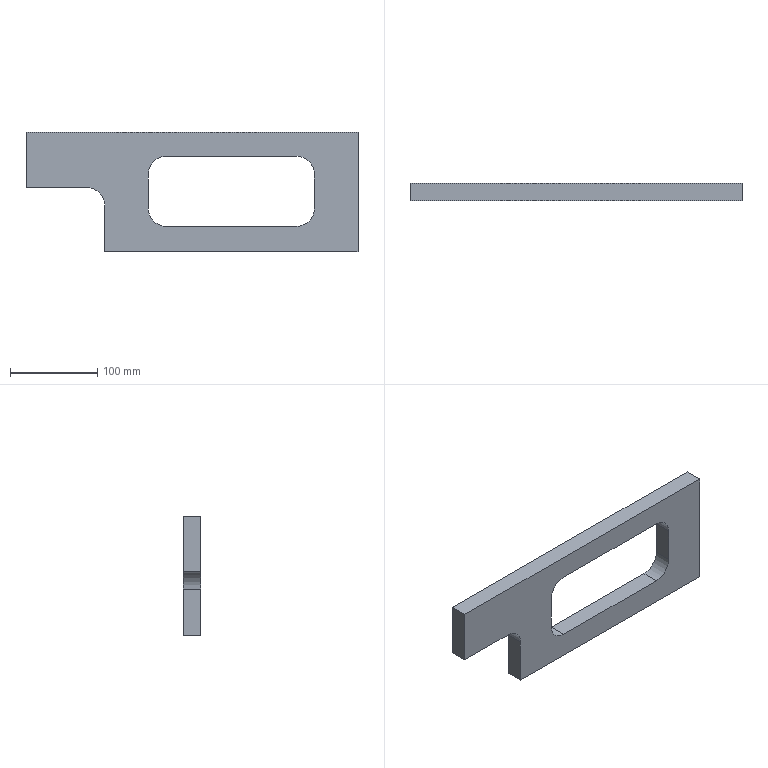Part | STEP file | Tube feed_id654_x_t | 1 solid | 17 faces | box 380 x 20 x 137 mm | volume 613484 mm3 | plane 12 | cylinder 5 | commonest cylinder face diameters 40 x5
STEP:
#1=CARTESIAN_POINT('',(0.,0.,0.));
#2=DIRECTION('',(0.,0.,1.));
#3=DIRECTION('',(1.,0.,0.));
#4=AXIS2_PLACEMENT_3D('',#1,#2,#3);
#5=CARTESIAN_POINT('',(206.,331.936,-108.75));
#6=VERTEX_POINT('',#5);
#7=CARTESIAN_POINT('',(206.,331.936,-68.75));
#8=VERTEX_POINT('',#7);
#9=CARTESIAN_POINT('',(206.,331.936,-48.75));
#10=DIRECTION('',(0.,0.,1.));
#11=VECTOR('',#10,1.);
#12=LINE('',#9,#11);
#13=CARTESIAN_POINT('',(206.,351.936,-48.75));
#14=DIRECTION('',(1.,0.,0.));
#15=DIRECTION('',(0.,0.,-1.));
#16=AXIS2_PLACEMENT_3D('',#13,#14,#15);
#17=PLANE('',#16);
#18=CARTESIAN_POINT('',(0.,-20.));
#19=DIRECTION('',(-1.,0.));
#20=VECTOR('',#19,1.);
#21=LINE('',#18,#20);
#22=(GEOMETRIC_REPRESENTATION_CONTEXT(2)PARAMETRIC_REPRESENTATION_CONTEXT()REPRESENTATION_CONTEXT('',''));
#23=DEFINITIONAL_REPRESENTATION('',(#21),#22);
#24=PCURVE('',#17,#23);
#25=CARTESIAN_POINT('',(0.,331.936,0.));
#26=DIRECTION('',(0.,-1.,0.));
#27=DIRECTION('',(0.,0.,1.));
#28=AXIS2_PLACEMENT_3D('',#25,#26,#27);
#29=PLANE('',#28);
#30=CARTESIAN_POINT('',(-48.75,-206.));
#31=DIRECTION('',(1.,0.));
#32=VECTOR('',#31,1.);
#33=LINE('',#30,#32);
#34=(GEOMETRIC_REPRESENTATION_CONTEXT(2)PARAMETRIC_REPRESENTATION_CONTEXT()REPRESENTATION_CONTEXT('',''));
#35=DEFINITIONAL_REPRESENTATION('',(#33),#34);
#36=PCURVE('',#29,#35);
#37=SURFACE_CURVE('',#12,(#24,#36),.PCURVE_S1.);
#38=EDGE_CURVE('',#6,#8,#37,.T.);
#39=ORIENTED_EDGE('',*,*,#38,.F.);
#40=CARTESIAN_POINT('',(206.,351.936,-108.75));
#41=VERTEX_POINT('',#40);
#42=CARTESIAN_POINT('',(206.,331.936,-108.75));
#43=DIRECTION('',(0.,1.,0.));
#44=VECTOR('',#43,1.);
#45=LINE('',#42,#44);
#46=CARTESIAN_POINT('',(60.,-20.));
#47=DIRECTION('',(0.,1.));
#48=VECTOR('',#47,1.);
#49=LINE('',#46,#48);
#50=(GEOMETRIC_REPRESENTATION_CONTEXT(2)PARAMETRIC_REPRESENTATION_CONTEXT()REPRESENTATION_CONTEXT('',''));
#51=DEFINITIONAL_REPRESENTATION('',(#49),#50);
#52=PCURVE('',#17,#51);
#53=CARTESIAN_POINT('',(226.,351.936,-108.75));
#54=DIRECTION('',(0.,1.,0.));
#55=DIRECTION('',(0.,0.,-1.));
#56=AXIS2_PLACEMENT_3D('',#53,#54,#55);
#57=CYLINDRICAL_SURFACE('',#56,20.);
#58=CARTESIAN_POINT('',(1.571,-20.));
#59=DIRECTION('',(0.,1.));
#60=VECTOR('',#59,1.);
#61=LINE('',#58,#60);
#62=(GEOMETRIC_REPRESENTATION_CONTEXT(2)PARAMETRIC_REPRESENTATION_CONTEXT()REPRESENTATION_CONTEXT('',''));
#63=DEFINITIONAL_REPRESENTATION('',(#61),#62);
#64=PCURVE('',#57,#63);
#65=SURFACE_CURVE('',#45,(#52,#64),.PCURVE_S1.);
#66=EDGE_CURVE('',#6,#41,#65,.T.);
#67=ORIENTED_EDGE('',*,*,#66,.T.);
#68=CARTESIAN_POINT('',(206.,351.936,-68.75));
#69=VERTEX_POINT('',#68);
#70=CARTESIAN_POINT('',(206.,351.936,-48.75));
#71=DIRECTION('',(0.,0.,1.));
#72=VECTOR('',#71,1.);
#73=LINE('',#70,#72);
#74=CARTESIAN_POINT('',(0.,0.));
#75=DIRECTION('',(-1.,0.));
#76=VECTOR('',#75,1.);
#77=LINE('',#74,#76);
#78=(GEOMETRIC_REPRESENTATION_CONTEXT(2)PARAMETRIC_REPRESENTATION_CONTEXT()REPRESENTATION_CONTEXT('',''));
#79=DEFINITIONAL_REPRESENTATION('',(#77),#78);
#80=PCURVE('',#17,#79);
#81=CARTESIAN_POINT('',(0.,351.936,0.));
#82=DIRECTION('',(0.,-1.,0.));
#83=DIRECTION('',(0.,0.,1.));
#84=AXIS2_PLACEMENT_3D('',#81,#82,#83);
#85=PLANE('',#84);
#86=CARTESIAN_POINT('',(-48.75,-206.));
#87=DIRECTION('',(1.,0.));
#88=VECTOR('',#87,1.);
#89=LINE('',#86,#88);
#90=(GEOMETRIC_REPRESENTATION_CONTEXT(2)PARAMETRIC_REPRESENTATION_CONTEXT()REPRESENTATION_CONTEXT('',''));
#91=DEFINITIONAL_REPRESENTATION('',(#89),#90);
#92=PCURVE('',#85,#91);
#93=SURFACE_CURVE('',#73,(#80,#92),.PCURVE_S1.);
#94=EDGE_CURVE('',#41,#69,#93,.T.);
#95=ORIENTED_EDGE('',*,*,#94,.T.);
#96=CARTESIAN_POINT('',(206.,351.936,-68.75));
#97=DIRECTION('',(0.,-1.,0.));
#98=VECTOR('',#97,1.);
#99=LINE('',#96,#98);
#100=CARTESIAN_POINT('',(20.,0.));
#101=DIRECTION('',(0.,-1.));
#102=VECTOR('',#101,1.);
#103=LINE('',#100,#102);
#104=(GEOMETRIC_REPRESENTATION_CONTEXT(2)PARAMETRIC_REPRESENTATION_CONTEXT()REPRESENTATION_CONTEXT('',''));
#105=DEFINITIONAL_REPRESENTATION('',(#103),#104);
#106=PCURVE('',#17,#105);
#107=CARTESIAN_POINT('',(226.,351.936,-68.75));
#108=DIRECTION('',(0.,1.,0.));
#109=DIRECTION('',(0.,0.,-1.));
#110=AXIS2_PLACEMENT_3D('',#107,#108,#109);
#111=CYLINDRICAL_SURFACE('',#110,20.);
#112=CARTESIAN_POINT('',(1.571,0.));
#113=DIRECTION('',(0.,-1.));
#114=VECTOR('',#113,1.);
#115=LINE('',#112,#114);
#116=(GEOMETRIC_REPRESENTATION_CONTEXT(2)PARAMETRIC_REPRESENTATION_CONTEXT()REPRESENTATION_CONTEXT('',''));
#117=DEFINITIONAL_REPRESENTATION('',(#115),#116);
#118=PCURVE('',#111,#117);
#119=SURFACE_CURVE('',#99,(#106,#118),.PCURVE_S1.);
#120=EDGE_CURVE('',#69,#8,#119,.T.);
#121=ORIENTED_EDGE('',*,*,#120,.T.);
#122=EDGE_LOOP('',(#39,#67,#95,#121));
#123=FACE_BOUND('',#122,.T.);
#124=ADVANCED_FACE('',(#123),#17,.T.);
#125=CARTESIAN_POINT('',(376.,351.936,-128.75));
#126=VERTEX_POINT('',#125);
#127=CARTESIAN_POINT('',(226.,351.936,-128.75));
#128=VERTEX_POINT('',#127);
#129=CARTESIAN_POINT('',(206.,351.936,-128.75));
#130=DIRECTION('',(-1.,0.,0.));
#131=VECTOR('',#130,1.);
#132=LINE('',#129,#131);
#133=CARTESIAN_POINT('',(206.,351.936,-128.75));
#134=DIRECTION('',(0.,0.,1.));
#135=DIRECTION('',(1.,0.,0.));
#136=AXIS2_PLACEMENT_3D('',#133,#134,#135);
#137=PLANE('',#136);
#138=CARTESIAN_POINT('',(0.,0.));
#139=DIRECTION('',(-1.,0.));
#140=VECTOR('',#139,1.);
#141=LINE('',#138,#140);
#142=(GEOMETRIC_REPRESENTATION_CONTEXT(2)PARAMETRIC_REPRESENTATION_CONTEXT()REPRESENTATION_CONTEXT('',''));
#143=DEFINITIONAL_REPRESENTATION('',(#141),#142);
#144=PCURVE('',#137,#143);
#145=CARTESIAN_POINT('',(-128.75,-206.));
#146=DIRECTION('',(0.,1.));
#147=VECTOR('',#146,1.);
#148=LINE('',#145,#147);
#149=(GEOMETRIC_REPRESENTATION_CONTEXT(2)PARAMETRIC_REPRESENTATION_CONTEXT()REPRESENTATION_CONTEXT('',''));
#150=DEFINITIONAL_REPRESENTATION('',(#148),#149);
#151=PCURVE('',#85,#150);
#152=SURFACE_CURVE('',#132,(#144,#151),.PCURVE_S1.);
#153=EDGE_CURVE('',#126,#128,#152,.T.);
#154=ORIENTED_EDGE('',*,*,#153,.T.);
#155=CARTESIAN_POINT('',(226.,331.936,-128.75));
#156=VERTEX_POINT('',#155);
#157=CARTESIAN_POINT('',(226.,351.936,-128.75));
#158=DIRECTION('',(0.,-1.,0.));
#159=VECTOR('',#158,1.);
#160=LINE('',#157,#159);
#161=CARTESIAN_POINT('',(20.,0.));
#162=DIRECTION('',(0.,-1.));
#163=VECTOR('',#162,1.);
#164=LINE('',#161,#163);
#165=(GEOMETRIC_REPRESENTATION_CONTEXT(2)PARAMETRIC_REPRESENTATION_CONTEXT()REPRESENTATION_CONTEXT('',''));
#166=DEFINITIONAL_REPRESENTATION('',(#164),#165);
#167=PCURVE('',#137,#166);
#168=CARTESIAN_POINT('',(0.,0.));
#169=DIRECTION('',(0.,-1.));
#170=VECTOR('',#169,1.);
#171=LINE('',#168,#170);
#172=(GEOMETRIC_REPRESENTATION_CONTEXT(2)PARAMETRIC_REPRESENTATION_CONTEXT()REPRESENTATION_CONTEXT('',''));
#173=DEFINITIONAL_REPRESENTATION('',(#171),#172);
#174=PCURVE('',#57,#173);
#175=SURFACE_CURVE('',#160,(#167,#174),.PCURVE_S1.);
#176=EDGE_CURVE('',#128,#156,#175,.T.);
#177=ORIENTED_EDGE('',*,*,#176,.T.);
#178=CARTESIAN_POINT('',(376.,331.936,-128.75));
#179=VERTEX_POINT('',#178);
#180=CARTESIAN_POINT('',(206.,331.936,-128.75));
#181=DIRECTION('',(-1.,0.,0.));
#182=VECTOR('',#181,1.);
#183=LINE('',#180,#182);
#184=CARTESIAN_POINT('',(0.,-20.));
#185=DIRECTION('',(-1.,0.));
#186=VECTOR('',#185,1.);
#187=LINE('',#184,#186);
#188=(GEOMETRIC_REPRESENTATION_CONTEXT(2)PARAMETRIC_REPRESENTATION_CONTEXT()REPRESENTATION_CONTEXT('',''));
#189=DEFINITIONAL_REPRESENTATION('',(#187),#188);
#190=PCURVE('',#137,#189);
#191=CARTESIAN_POINT('',(-128.75,-206.));
#192=DIRECTION('',(0.,1.));
#193=VECTOR('',#192,1.);
#194=LINE('',#191,#193);
#195=(GEOMETRIC_REPRESENTATION_CONTEXT(2)PARAMETRIC_REPRESENTATION_CONTEXT()REPRESENTATION_CONTEXT('',''));
#196=DEFINITIONAL_REPRESENTATION('',(#194),#195);
#197=PCURVE('',#29,#196);
#198=SURFACE_CURVE('',#183,(#190,#197),.PCURVE_S1.);
#199=EDGE_CURVE('',#179,#156,#198,.T.);
#200=ORIENTED_EDGE('',*,*,#199,.F.);
#201=CARTESIAN_POINT('',(376.,331.936,-128.75));
#202=DIRECTION('',(0.,1.,0.));
#203=VECTOR('',#202,1.);
#204=LINE('',#201,#203);
#205=CARTESIAN_POINT('',(170.,-20.));
#206=DIRECTION('',(0.,1.));
#207=VECTOR('',#206,1.);
#208=LINE('',#205,#207);
#209=(GEOMETRIC_REPRESENTATION_CONTEXT(2)PARAMETRIC_REPRESENTATION_CONTEXT()REPRESENTATION_CONTEXT('',''));
#210=DEFINITIONAL_REPRESENTATION('',(#208),#209);
#211=PCURVE('',#137,#210);
#212=CARTESIAN_POINT('',(376.,351.936,-108.75));
#213=DIRECTION('',(0.,1.,0.));
#214=DIRECTION('',(0.,0.,-1.));
#215=AXIS2_PLACEMENT_3D('',#212,#213,#214);
#216=CYLINDRICAL_SURFACE('',#215,20.);
#217=CARTESIAN_POINT('',(6.283,-20.));
#218=DIRECTION('',(0.,1.));
#219=VECTOR('',#218,1.);
#220=LINE('',#217,#219);
#221=(GEOMETRIC_REPRESENTATION_CONTEXT(2)PARAMETRIC_REPRESENTATION_CONTEXT()REPRESENTATION_CONTEXT('',''));
#222=DEFINITIONAL_REPRESENTATION('',(#220),#221);
#223=PCURVE('',#216,#222);
#224=SURFACE_CURVE('',#204,(#211,#223),.PCURVE_S1.);
#225=EDGE_CURVE('',#179,#126,#224,.T.);
#226=ORIENTED_EDGE('',*,*,#225,.T.);
#227=EDGE_LOOP('',(#154,#177,#200,#226));
#228=FACE_BOUND('',#227,.T.);
#229=ADVANCED_FACE('',(#228),#137,.T.);
#230=CARTESIAN_POINT('',(396.,331.936,-68.75));
#231=VERTEX_POINT('',#230);
#232=CARTESIAN_POINT('',(396.,331.936,-108.75));
#233=VERTEX_POINT('',#232);
#234=CARTESIAN_POINT('',(396.,331.936,-128.75));
#235=DIRECTION('',(0.,0.,-1.));
#236=VECTOR('',#235,1.);
#237=LINE('',#234,#236);
#238=CARTESIAN_POINT('',(396.,351.936,-128.75));
#239=DIRECTION('',(-1.,0.,0.));
#240=DIRECTION('',(0.,0.,1.));
#241=AXIS2_PLACEMENT_3D('',#238,#239,#240);
#242=PLANE('',#241);
#243=CARTESIAN_POINT('',(0.,-20.));
#244=DIRECTION('',(-1.,0.));
#245=VECTOR('',#244,1.);
#246=LINE('',#243,#245);
#247=(GEOMETRIC_REPRESENTATION_CONTEXT(2)PARAMETRIC_REPRESENTATION_CONTEXT()REPRESENTATION_CONTEXT('',''));
#248=DEFINITIONAL_REPRESENTATION('',(#246),#247);
#249=PCURVE('',#242,#248);
#250=CARTESIAN_POINT('',(-128.75,-396.));
#251=DIRECTION('',(-1.,0.));
#252=VECTOR('',#251,1.);
#253=LINE('',#250,#252);
#254=(GEOMETRIC_REPRESENTATION_CONTEXT(2)PARAMETRIC_REPRESENTATION_CONTEXT()REPRESENTATION_CONTEXT('',''));
#255=DEFINITIONAL_REPRESENTATION('',(#253),#254);
#256=PCURVE('',#29,#255);
#257=SURFACE_CURVE('',#237,(#249,#256),.PCURVE_S1.);
#258=EDGE_CURVE('',#231,#233,#257,.T.);
#259=ORIENTED_EDGE('',*,*,#258,.F.);
#260=CARTESIAN_POINT('',(396.,351.936,-68.75));
#261=VERTEX_POINT('',#260);
#262=CARTESIAN_POINT('',(396.,331.936,-68.75));
#263=DIRECTION('',(0.,1.,0.));
#264=VECTOR('',#263,1.);
#265=LINE('',#262,#264);
#266=CARTESIAN_POINT('',(60.,-20.));
#267=DIRECTION('',(0.,1.));
#268=VECTOR('',#267,1.);
#269=LINE('',#266,#268);
#270=(GEOMETRIC_REPRESENTATION_CONTEXT(2)PARAMETRIC_REPRESENTATION_CONTEXT()REPRESENTATION_CONTEXT('',''));
#271=DEFINITIONAL_REPRESENTATION('',(#269),#270);
#272=PCURVE('',#242,#271);
#273=CARTESIAN_POINT('',(376.,351.936,-68.75));
#274=DIRECTION('',(0.,1.,0.));
#275=DIRECTION('',(0.,0.,-1.));
#276=AXIS2_PLACEMENT_3D('',#273,#274,#275);
#277=CYLINDRICAL_SURFACE('',#276,20.);
#278=CARTESIAN_POINT('',(4.712,-20.));
#279=DIRECTION('',(0.,1.));
#280=VECTOR('',#279,1.);
#281=LINE('',#278,#280);
#282=(GEOMETRIC_REPRESENTATION_CONTEXT(2)PARAMETRIC_REPRESENTATION_CONTEXT()REPRESENTATION_CONTEXT('',''));
#283=DEFINITIONAL_REPRESENTATION('',(#281),#282);
#284=PCURVE('',#277,#283);
#285=SURFACE_CURVE('',#265,(#272,#284),.PCURVE_S1.);
#286=EDGE_CURVE('',#231,#261,#285,.T.);
#287=ORIENTED_EDGE('',*,*,#286,.T.);
#288=CARTESIAN_POINT('',(396.,351.936,-108.75));
#289=VERTEX_POINT('',#288);
#290=CARTESIAN_POINT('',(396.,351.936,-128.75));
#291=DIRECTION('',(0.,0.,-1.));
#292=VECTOR('',#291,1.);
#293=LINE('',#290,#292);
#294=CARTESIAN_POINT('',(0.,0.));
#295=DIRECTION('',(-1.,0.));
#296=VECTOR('',#295,1.);
#297=LINE('',#294,#296);
#298=(GEOMETRIC_REPRESENTATION_CONTEXT(2)PARAMETRIC_REPRESENTATION_CONTEXT()REPRESENTATION_CONTEXT('',''));
#299=DEFINITIONAL_REPRESENTATION('',(#297),#298);
#300=PCURVE('',#242,#299);
#301=CARTESIAN_POINT('',(-128.75,-396.));
#302=DIRECTION('',(-1.,0.));
#303=VECTOR('',#302,1.);
#304=LINE('',#301,#303);
#305=(GEOMETRIC_REPRESENTATION_CONTEXT(2)PARAMETRIC_REPRESENTATION_CONTEXT()REPRESENTATION_CONTEXT('',''));
#306=DEFINITIONAL_REPRESENTATION('',(#304),#305);
#307=PCURVE('',#85,#306);
#308=SURFACE_CURVE('',#293,(#300,#307),.PCURVE_S1.);
#309=EDGE_CURVE('',#261,#289,#308,.T.);
#310=ORIENTED_EDGE('',*,*,#309,.T.);
#311=CARTESIAN_POINT('',(396.,351.936,-108.75));
#312=DIRECTION('',(0.,-1.,0.));
#313=VECTOR('',#312,1.);
#314=LINE('',#311,#313);
#315=CARTESIAN_POINT('',(20.,0.));
#316=DIRECTION('',(0.,-1.));
#317=VECTOR('',#316,1.);
#318=LINE('',#315,#317);
#319=(GEOMETRIC_REPRESENTATION_CONTEXT(2)PARAMETRIC_REPRESENTATION_CONTEXT()REPRESENTATION_CONTEXT('',''));
#320=DEFINITIONAL_REPRESENTATION('',(#318),#319);
#321=PCURVE('',#242,#320);
#322=CARTESIAN_POINT('',(4.712,0.));
#323=DIRECTION('',(0.,-1.));
#324=VECTOR('',#323,1.);
#325=LINE('',#322,#324);
#326=(GEOMETRIC_REPRESENTATION_CONTEXT(2)PARAMETRIC_REPRESENTATION_CONTEXT()REPRESENTATION_CONTEXT('',''));
#327=DEFINITIONAL_REPRESENTATION('',(#325),#326);
#328=PCURVE('',#216,#327);
#329=SURFACE_CURVE('',#314,(#321,#328),.PCURVE_S1.);
#330=EDGE_CURVE('',#289,#233,#329,.T.);
#331=ORIENTED_EDGE('',*,*,#330,.T.);
#332=EDGE_LOOP('',(#259,#287,#310,#331));
#333=FACE_BOUND('',#332,.T.);
#334=ADVANCED_FACE('',(#333),#242,.T.);
#335=CARTESIAN_POINT('',(66.,331.936,-21.));
#336=VERTEX_POINT('',#335);
#337=CARTESIAN_POINT('',(66.,331.936,-84.5));
#338=VERTEX_POINT('',#337);
#339=CARTESIAN_POINT('',(66.,331.936,-84.5));
#340=DIRECTION('',(0.,0.,-1.));
#341=VECTOR('',#340,1.);
#342=LINE('',#339,#341);
#343=CARTESIAN_POINT('',(66.,351.936,-84.5));
#344=DIRECTION('',(-1.,0.,0.));
#345=DIRECTION('',(0.,0.,1.));
#346=AXIS2_PLACEMENT_3D('',#343,#344,#345);
#347=PLANE('',#346);
#348=CARTESIAN_POINT('',(0.,-20.));
#349=DIRECTION('',(-1.,0.));
#350=VECTOR('',#349,1.);
#351=LINE('',#348,#350);
#352=(GEOMETRIC_REPRESENTATION_CONTEXT(2)PARAMETRIC_REPRESENTATION_CONTEXT()REPRESENTATION_CONTEXT('',''));
#353=DEFINITIONAL_REPRESENTATION('',(#351),#352);
#354=PCURVE('',#347,#353);
#355=CARTESIAN_POINT('',(-84.5,-66.));
#356=DIRECTION('',(-1.,0.));
#357=VECTOR('',#356,1.);
#358=LINE('',#355,#357);
#359=(GEOMETRIC_REPRESENTATION_CONTEXT(2)PARAMETRIC_REPRESENTATION_CONTEXT()REPRESENTATION_CONTEXT('',''));
#360=DEFINITIONAL_REPRESENTATION('',(#358),#359);
#361=PCURVE('',#29,#360);
#362=SURFACE_CURVE('',#342,(#354,#361),.PCURVE_S1.);
#363=EDGE_CURVE('',#336,#338,#362,.T.);
#364=ORIENTED_EDGE('',*,*,#363,.F.);
#365=CARTESIAN_POINT('',(66.,351.936,-21.));
#366=VERTEX_POINT('',#365);
#367=CARTESIAN_POINT('',(66.,351.936,-21.));
#368=DIRECTION('',(0.,1.,0.));
#369=VECTOR('',#368,1.);
#370=LINE('',#367,#369);
#371=CARTESIAN_POINT('',(63.5,0.));
#372=DIRECTION('',(0.,1.));
#373=VECTOR('',#372,1.);
#374=LINE('',#371,#373);
#375=(GEOMETRIC_REPRESENTATION_CONTEXT(2)PARAMETRIC_REPRESENTATION_CONTEXT()REPRESENTATION_CONTEXT('',''));
#376=DEFINITIONAL_REPRESENTATION('',(#374),#375);
#377=PCURVE('',#347,#376);
#378=CARTESIAN_POINT('',(66.,351.936,-21.));
#379=DIRECTION('',(0.,0.,1.));
#380=DIRECTION('',(1.,0.,0.));
#381=AXIS2_PLACEMENT_3D('',#378,#379,#380);
#382=PLANE('',#381);
#383=CARTESIAN_POINT('',(0.,0.));
#384=DIRECTION('',(0.,1.));
#385=VECTOR('',#384,1.);
#386=LINE('',#383,#385);
#387=(GEOMETRIC_REPRESENTATION_CONTEXT(2)PARAMETRIC_REPRESENTATION_CONTEXT()REPRESENTATION_CONTEXT('',''));
#388=DEFINITIONAL_REPRESENTATION('',(#386),#387);
#389=PCURVE('',#382,#388);
#390=SURFACE_CURVE('',#370,(#377,#389),.PCURVE_S1.);
#391=EDGE_CURVE('',#336,#366,#390,.T.);
#392=ORIENTED_EDGE('',*,*,#391,.T.);
#393=CARTESIAN_POINT('',(66.,351.936,-84.5));
#394=VERTEX_POINT('',#393);
#395=CARTESIAN_POINT('',(66.,351.936,-84.5));
#396=DIRECTION('',(0.,0.,-1.));
#397=VECTOR('',#396,1.);
#398=LINE('',#395,#397);
#399=CARTESIAN_POINT('',(0.,0.));
#400=DIRECTION('',(-1.,0.));
#401=VECTOR('',#400,1.);
#402=LINE('',#399,#401);
#403=(GEOMETRIC_REPRESENTATION_CONTEXT(2)PARAMETRIC_REPRESENTATION_CONTEXT()REPRESENTATION_CONTEXT('',''));
#404=DEFINITIONAL_REPRESENTATION('',(#402),#403);
#405=PCURVE('',#347,#404);
#406=CARTESIAN_POINT('',(-84.5,-66.));
#407=DIRECTION('',(-1.,0.));
#408=VECTOR('',#407,1.);
#409=LINE('',#406,#408);
#410=(GEOMETRIC_REPRESENTATION_CONTEXT(2)PARAMETRIC_REPRESENTATION_CONTEXT()REPRESENTATION_CONTEXT('',''));
#411=DEFINITIONAL_REPRESENTATION('',(#409),#410);
#412=PCURVE('',#85,#411);
#413=SURFACE_CURVE('',#398,(#405,#412),.PCURVE_S1.);
#414=EDGE_CURVE('',#366,#394,#413,.T.);
#415=ORIENTED_EDGE('',*,*,#414,.T.);
#416=CARTESIAN_POINT('',(66.,351.936,-84.5));
#417=DIRECTION('',(0.,1.,0.));
#418=VECTOR('',#417,1.);
#419=LINE('',#416,#418);
#420=CARTESIAN_POINT('',(0.,0.));
#421=DIRECTION('',(0.,1.));
#422=VECTOR('',#421,1.);
#423=LINE('',#420,#422);
#424=(GEOMETRIC_REPRESENTATION_CONTEXT(2)PARAMETRIC_REPRESENTATION_CONTEXT()REPRESENTATION_CONTEXT('',''));
#425=DEFINITIONAL_REPRESENTATION('',(#423),#424);
#426=PCURVE('',#347,#425);
#427=CARTESIAN_POINT('',(156.,351.936,-84.5));
#428=DIRECTION('',(0.,0.,-1.));
#429=DIRECTION('',(-1.,0.,0.));
#430=AXIS2_PLACEMENT_3D('',#427,#428,#429);
#431=PLANE('',#430);
#432=CARTESIAN_POINT('',(90.,0.));
#433=DIRECTION('',(0.,1.));
#434=VECTOR('',#433,1.);
#435=LINE('',#432,#434);
#436=(GEOMETRIC_REPRESENTATION_CONTEXT(2)PARAMETRIC_REPRESENTATION_CONTEXT()REPRESENTATION_CONTEXT('',''));
#437=DEFINITIONAL_REPRESENTATION('',(#435),#436);
#438=PCURVE('',#431,#437);
#439=SURFACE_CURVE('',#419,(#426,#438),.PCURVE_S1.);
#440=EDGE_CURVE('',#338,#394,#439,.T.);
#441=ORIENTED_EDGE('',*,*,#440,.F.);
#442=EDGE_LOOP('',(#364,#392,#415,#441));
#443=FACE_BOUND('',#442,.T.);
#444=ADVANCED_FACE('',(#443),#347,.T.);
#445=CARTESIAN_POINT('',(446.,331.936,-21.));
#446=VERTEX_POINT('',#445);
#447=CARTESIAN_POINT('',(0.,331.936,-21.));
#448=DIRECTION('',(-1.,0.,0.));
#449=VECTOR('',#448,1.);
#450=LINE('',#447,#449);
#451=CARTESIAN_POINT('',(-66.,-20.));
#452=DIRECTION('',(-1.,0.));
#453=VECTOR('',#452,1.);
#454=LINE('',#451,#453);
#455=(GEOMETRIC_REPRESENTATION_CONTEXT(2)PARAMETRIC_REPRESENTATION_CONTEXT()REPRESENTATION_CONTEXT('',''));
#456=DEFINITIONAL_REPRESENTATION('',(#454),#455);
#457=PCURVE('',#382,#456);
#458=CARTESIAN_POINT('',(-21.,0.));
#459=DIRECTION('',(0.,1.));
#460=VECTOR('',#459,1.);
#461=LINE('',#458,#460);
#462=(GEOMETRIC_REPRESENTATION_CONTEXT(2)PARAMETRIC_REPRESENTATION_CONTEXT()REPRESENTATION_CONTEXT('',''));
#463=DEFINITIONAL_REPRESENTATION('',(#461),#462);
#464=PCURVE('',#29,#463);
#465=SURFACE_CURVE('',#450,(#457,#464),.PCURVE_S1.);
#466=EDGE_CURVE('',#446,#336,#465,.T.);
#467=ORIENTED_EDGE('',*,*,#466,.F.);
#468=CARTESIAN_POINT('',(446.,351.936,-21.));
#469=VERTEX_POINT('',#468);
#470=CARTESIAN_POINT('',(446.,351.936,-21.));
#471=DIRECTION('',(0.,1.,0.));
#472=VECTOR('',#471,1.);
#473=LINE('',#470,#472);
#474=CARTESIAN_POINT('',(380.,0.));
#475=DIRECTION('',(0.,1.));
#476=VECTOR('',#475,1.);
#477=LINE('',#474,#476);
#478=(GEOMETRIC_REPRESENTATION_CONTEXT(2)PARAMETRIC_REPRESENTATION_CONTEXT()REPRESENTATION_CONTEXT('',''));
#479=DEFINITIONAL_REPRESENTATION('',(#477),#478);
#480=PCURVE('',#382,#479);
#481=CARTESIAN_POINT('',(446.,351.936,-19.5));
#482=DIRECTION('',(1.,0.,0.));
#483=DIRECTION('',(0.,0.,-1.));
#484=AXIS2_PLACEMENT_3D('',#481,#482,#483);
#485=PLANE('',#484);
#486=CARTESIAN_POINT('',(1.5,0.));
#487=DIRECTION('',(0.,1.));
#488=VECTOR('',#487,1.);
#489=LINE('',#486,#488);
#490=(GEOMETRIC_REPRESENTATION_CONTEXT(2)PARAMETRIC_REPRESENTATION_CONTEXT()REPRESENTATION_CONTEXT('',''));
#491=DEFINITIONAL_REPRESENTATION('',(#489),#490);
#492=PCURVE('',#485,#491);
#493=SURFACE_CURVE('',#473,(#480,#492),.PCURVE_S1.);
#494=EDGE_CURVE('',#446,#469,#493,.T.);
#495=ORIENTED_EDGE('',*,*,#494,.T.);
#496=CARTESIAN_POINT('',(0.,351.936,-21.));
#497=DIRECTION('',(-1.,0.,0.));
#498=VECTOR('',#497,1.);
#499=LINE('',#496,#498);
#500=CARTESIAN_POINT('',(-66.,0.));
#501=DIRECTION('',(-1.,0.));
#502=VECTOR('',#501,1.);
#503=LINE('',#500,#502);
#504=(GEOMETRIC_REPRESENTATION_CONTEXT(2)PARAMETRIC_REPRESENTATION_CONTEXT()REPRESENTATION_CONTEXT('',''));
#505=DEFINITIONAL_REPRESENTATION('',(#503),#504);
#506=PCURVE('',#382,#505);
#507=CARTESIAN_POINT('',(-21.,0.));
#508=DIRECTION('',(0.,1.));
#509=VECTOR('',#508,1.);
#510=LINE('',#507,#509);
#511=(GEOMETRIC_REPRESENTATION_CONTEXT(2)PARAMETRIC_REPRESENTATION_CONTEXT()REPRESENTATION_CONTEXT('',''));
#512=DEFINITIONAL_REPRESENTATION('',(#510),#511);
#513=PCURVE('',#85,#512);
#514=SURFACE_CURVE('',#499,(#506,#513),.PCURVE_S1.);
#515=EDGE_CURVE('',#469,#366,#514,.T.);
#516=ORIENTED_EDGE('',*,*,#515,.T.);
#517=ORIENTED_EDGE('',*,*,#391,.F.);
#518=EDGE_LOOP('',(#467,#495,#516,#517));
#519=FACE_BOUND('',#518,.T.);
#520=ADVANCED_FACE('',(#519),#382,.T.);
#521=CARTESIAN_POINT('',(446.,331.936,-158.));
#522=VERTEX_POINT('',#521);
#523=CARTESIAN_POINT('',(446.,331.936,-19.5));
#524=DIRECTION('',(0.,0.,1.));
#525=VECTOR('',#524,1.);
#526=LINE('',#523,#525);
#527=CARTESIAN_POINT('',(0.,-20.));
#528=DIRECTION('',(-1.,0.));
#529=VECTOR('',#528,1.);
#530=LINE('',#527,#529);
#531=(GEOMETRIC_REPRESENTATION_CONTEXT(2)PARAMETRIC_REPRESENTATION_CONTEXT()REPRESENTATION_CONTEXT('',''));
#532=DEFINITIONAL_REPRESENTATION('',(#530),#531);
#533=PCURVE('',#485,#532);
#534=CARTESIAN_POINT('',(-19.5,-446.));
#535=DIRECTION('',(1.,0.));
#536=VECTOR('',#535,1.);
#537=LINE('',#534,#536);
#538=(GEOMETRIC_REPRESENTATION_CONTEXT(2)PARAMETRIC_REPRESENTATION_CONTEXT()REPRESENTATION_CONTEXT('',''));
#539=DEFINITIONAL_REPRESENTATION('',(#537),#538);
#540=PCURVE('',#29,#539);
#541=SURFACE_CURVE('',#526,(#533,#540),.PCURVE_S1.);
#542=EDGE_CURVE('',#522,#446,#541,.T.);
#543=ORIENTED_EDGE('',*,*,#542,.F.);
#544=CARTESIAN_POINT('',(446.,351.936,-158.));
#545=VERTEX_POINT('',#544);
#546=CARTESIAN_POINT('',(446.,351.936,-158.));
#547=DIRECTION('',(0.,1.,0.));
#548=VECTOR('',#547,1.);
#549=LINE('',#546,#548);
#550=CARTESIAN_POINT('',(138.5,0.));
#551=DIRECTION('',(0.,1.));
#552=VECTOR('',#551,1.);
#553=LINE('',#550,#552);
#554=(GEOMETRIC_REPRESENTATION_CONTEXT(2)PARAMETRIC_REPRESENTATION_CONTEXT()REPRESENTATION_CONTEXT('',''));
#555=DEFINITIONAL_REPRESENTATION('',(#553),#554);
#556=PCURVE('',#485,#555);
#557=CARTESIAN_POINT('',(446.,351.936,-158.));
#558=DIRECTION('',(0.,0.,-1.));
#559=DIRECTION('',(-1.,0.,0.));
#560=AXIS2_PLACEMENT_3D('',#557,#558,#559);
#561=PLANE('',#560);
#562=CARTESIAN_POINT('',(0.,0.));
#563=DIRECTION('',(0.,1.));
#564=VECTOR('',#563,1.);
#565=LINE('',#562,#564);
#566=(GEOMETRIC_REPRESENTATION_CONTEXT(2)PARAMETRIC_REPRESENTATION_CONTEXT()REPRESENTATION_CONTEXT('',''));
#567=DEFINITIONAL_REPRESENTATION('',(#565),#566);
#568=PCURVE('',#561,#567);
#569=SURFACE_CURVE('',#549,(#556,#568),.PCURVE_S1.);
#570=EDGE_CURVE('',#522,#545,#569,.T.);
#571=ORIENTED_EDGE('',*,*,#570,.T.);
#572=CARTESIAN_POINT('',(446.,351.936,-19.5));
#573=DIRECTION('',(0.,0.,1.));
#574=VECTOR('',#573,1.);
#575=LINE('',#572,#574);
#576=CARTESIAN_POINT('',(0.,0.));
#577=DIRECTION('',(-1.,0.));
#578=VECTOR('',#577,1.);
#579=LINE('',#576,#578);
#580=(GEOMETRIC_REPRESENTATION_CONTEXT(2)PARAMETRIC_REPRESENTATION_CONTEXT()REPRESENTATION_CONTEXT('',''));
#581=DEFINITIONAL_REPRESENTATION('',(#579),#580);
#582=PCURVE('',#485,#581);
#583=CARTESIAN_POINT('',(-19.5,-446.));
#584=DIRECTION('',(1.,0.));
#585=VECTOR('',#584,1.);
#586=LINE('',#583,#585);
#587=(GEOMETRIC_REPRESENTATION_CONTEXT(2)PARAMETRIC_REPRESENTATION_CONTEXT()REPRESENTATION_CONTEXT('',''));
#588=DEFINITIONAL_REPRESENTATION('',(#586),#587);
#589=PCURVE('',#85,#588);
#590=SURFACE_CURVE('',#575,(#582,#589),.PCURVE_S1.);
#591=EDGE_CURVE('',#545,#469,#590,.T.);
#592=ORIENTED_EDGE('',*,*,#591,.T.);
#593=ORIENTED_EDGE('',*,*,#494,.F.);
#594=EDGE_LOOP('',(#543,#571,#592,#593));
#595=FACE_BOUND('',#594,.T.);
#596=ADVANCED_FACE('',(#595),#485,.T.);
#597=CARTESIAN_POINT('',(156.,331.936,-158.));
#598=VERTEX_POINT('',#597);
#599=CARTESIAN_POINT('',(446.,331.936,-158.));
#600=DIRECTION('',(1.,0.,0.));
#601=VECTOR('',#600,1.);
#602=LINE('',#599,#601);
#603=CARTESIAN_POINT('',(0.,-20.));
#604=DIRECTION('',(-1.,0.));
#605=VECTOR('',#604,1.);
#606=LINE('',#603,#605);
#607=(GEOMETRIC_REPRESENTATION_CONTEXT(2)PARAMETRIC_REPRESENTATION_CONTEXT()REPRESENTATION_CONTEXT('',''));
#608=DEFINITIONAL_REPRESENTATION('',(#606),#607);
#609=PCURVE('',#561,#608);
#610=CARTESIAN_POINT('',(-158.,-446.));
#611=DIRECTION('',(0.,-1.));
#612=VECTOR('',#611,1.);
#613=LINE('',#610,#612);
#614=(GEOMETRIC_REPRESENTATION_CONTEXT(2)PARAMETRIC_REPRESENTATION_CONTEXT()REPRESENTATION_CONTEXT('',''));
#615=DEFINITIONAL_REPRESENTATION('',(#613),#614);
#616=PCURVE('',#29,#615);
#617=SURFACE_CURVE('',#602,(#609,#616),.PCURVE_S1.);
#618=EDGE_CURVE('',#598,#522,#617,.T.);
#619=ORIENTED_EDGE('',*,*,#618,.F.);
#620=CARTESIAN_POINT('',(156.,351.936,-158.));
#621=VERTEX_POINT('',#620);
#622=CARTESIAN_POINT('',(156.,351.936,-158.));
#623=DIRECTION('',(0.,1.,0.));
#624=VECTOR('',#623,1.);
#625=LINE('',#622,#624);
#626=CARTESIAN_POINT('',(290.,0.));
#627=DIRECTION('',(0.,1.));
#628=VECTOR('',#627,1.);
#629=LINE('',#626,#628);
#630=(GEOMETRIC_REPRESENTATION_CONTEXT(2)PARAMETRIC_REPRESENTATION_CONTEXT()REPRESENTATION_CONTEXT('',''));
#631=DEFINITIONAL_REPRESENTATION('',(#629),#630);
#632=PCURVE('',#561,#631);
#633=CARTESIAN_POINT('',(156.,351.936,-158.));
#634=DIRECTION('',(-1.,0.,0.));
#635=DIRECTION('',(0.,0.,1.));
#636=AXIS2_PLACEMENT_3D('',#633,#634,#635);
#637=PLANE('',#636);
#638=CARTESIAN_POINT('',(0.,0.));
#639=DIRECTION('',(0.,1.));
#640=VECTOR('',#639,1.);
#641=LINE('',#638,#640);
#642=(GEOMETRIC_REPRESENTATION_CONTEXT(2)PARAMETRIC_REPRESENTATION_CONTEXT()REPRESENTATION_CONTEXT('',''));
#643=DEFINITIONAL_REPRESENTATION('',(#641),#642);
#644=PCURVE('',#637,#643);
#645=SURFACE_CURVE('',#625,(#632,#644),.PCURVE_S1.);
#646=EDGE_CURVE('',#598,#621,#645,.T.);
#647=ORIENTED_EDGE('',*,*,#646,.T.);
#648=CARTESIAN_POINT('',(446.,351.936,-158.));
#649=DIRECTION('',(1.,0.,0.));
#650=VECTOR('',#649,1.);
#651=LINE('',#648,#650);
#652=CARTESIAN_POINT('',(0.,0.));
#653=DIRECTION('',(-1.,0.));
#654=VECTOR('',#653,1.);
#655=LINE('',#652,#654);
#656=(GEOMETRIC_REPRESENTATION_CONTEXT(2)PARAMETRIC_REPRESENTATION_CONTEXT()REPRESENTATION_CONTEXT('',''));
#657=DEFINITIONAL_REPRESENTATION('',(#655),#656);
#658=PCURVE('',#561,#657);
#659=CARTESIAN_POINT('',(-158.,-446.));
#660=DIRECTION('',(0.,-1.));
#661=VECTOR('',#660,1.);
#662=LINE('',#659,#661);
#663=(GEOMETRIC_REPRESENTATION_CONTEXT(2)PARAMETRIC_REPRESENTATION_CONTEXT()REPRESENTATION_CONTEXT('',''));
#664=DEFINITIONAL_REPRESENTATION('',(#662),#663);
#665=PCURVE('',#85,#664);
#666=SURFACE_CURVE('',#651,(#658,#665),.PCURVE_S1.);
#667=EDGE_CURVE('',#621,#545,#666,.T.);
#668=ORIENTED_EDGE('',*,*,#667,.T.);
#669=ORIENTED_EDGE('',*,*,#570,.F.);
#670=EDGE_LOOP('',(#619,#647,#668,#669));
#671=FACE_BOUND('',#670,.T.);
#672=ADVANCED_FACE('',(#671),#561,.T.);
#673=CARTESIAN_POINT('',(156.,331.936,-104.5));
#674=VERTEX_POINT('',#673);
#675=CARTESIAN_POINT('',(156.,331.936,-158.));
#676=DIRECTION('',(0.,0.,-1.));
#677=VECTOR('',#676,1.);
#678=LINE('',#675,#677);
#679=CARTESIAN_POINT('',(0.,-20.));
#680=DIRECTION('',(-1.,0.));
#681=VECTOR('',#680,1.);
#682=LINE('',#679,#681);
#683=(GEOMETRIC_REPRESENTATION_CONTEXT(2)PARAMETRIC_REPRESENTATION_CONTEXT()REPRESENTATION_CONTEXT('',''));
#684=DEFINITIONAL_REPRESENTATION('',(#682),#683);
#685=PCURVE('',#637,#684);
#686=CARTESIAN_POINT('',(-158.,-156.));
#687=DIRECTION('',(-1.,0.));
#688=VECTOR('',#687,1.);
#689=LINE('',#686,#688);
#690=(GEOMETRIC_REPRESENTATION_CONTEXT(2)PARAMETRIC_REPRESENTATION_CONTEXT()REPRESENTATION_CONTEXT('',''));
#691=DEFINITIONAL_REPRESENTATION('',(#689),#690);
#692=PCURVE('',#29,#691);
#693=SURFACE_CURVE('',#678,(#685,#692),.PCURVE_S1.);
#694=EDGE_CURVE('',#674,#598,#693,.T.);
#695=ORIENTED_EDGE('',*,*,#694,.F.);
#696=CARTESIAN_POINT('',(156.,351.936,-104.5));
#697=VERTEX_POINT('',#696);
#698=CARTESIAN_POINT('',(156.,351.936,-104.5));
#699=DIRECTION('',(0.,1.,0.));
#700=VECTOR('',#699,1.);
#701=LINE('',#698,#700);
#702=CARTESIAN_POINT('',(53.5,0.));
#703=DIRECTION('',(0.,1.));
#704=VECTOR('',#703,1.);
#705=LINE('',#702,#704);
#706=(GEOMETRIC_REPRESENTATION_CONTEXT(2)PARAMETRIC_REPRESENTATION_CONTEXT()REPRESENTATION_CONTEXT('',''));
#707=DEFINITIONAL_REPRESENTATION('',(#705),#706);
#708=PCURVE('',#637,#707);
#709=CARTESIAN_POINT('',(136.,351.936,-104.5));
#710=DIRECTION('',(0.,-1.,0.));
#711=DIRECTION('',(0.,0.,-1.));
#712=AXIS2_PLACEMENT_3D('',#709,#710,#711);
#713=CYLINDRICAL_SURFACE('',#712,20.);
#714=CARTESIAN_POINT('',(1.571,0.));
#715=DIRECTION('',(0.,-1.));
#716=VECTOR('',#715,1.);
#717=LINE('',#714,#716);
#718=(GEOMETRIC_REPRESENTATION_CONTEXT(2)PARAMETRIC_REPRESENTATION_CONTEXT()REPRESENTATION_CONTEXT('',''));
#719=DEFINITIONAL_REPRESENTATION('',(#717),#718);
#720=PCURVE('',#713,#719);
#721=SURFACE_CURVE('',#701,(#708,#720),.PCURVE_S1.);
#722=EDGE_CURVE('',#674,#697,#721,.T.);
#723=ORIENTED_EDGE('',*,*,#722,.T.);
#724=CARTESIAN_POINT('',(156.,351.936,-158.));
#725=DIRECTION('',(0.,0.,-1.));
#726=VECTOR('',#725,1.);
#727=LINE('',#724,#726);
#728=CARTESIAN_POINT('',(0.,0.));
#729=DIRECTION('',(-1.,0.));
#730=VECTOR('',#729,1.);
#731=LINE('',#728,#730);
#732=(GEOMETRIC_REPRESENTATION_CONTEXT(2)PARAMETRIC_REPRESENTATION_CONTEXT()REPRESENTATION_CONTEXT('',''));
#733=DEFINITIONAL_REPRESENTATION('',(#731),#732);
#734=PCURVE('',#637,#733);
#735=CARTESIAN_POINT('',(-158.,-156.));
#736=DIRECTION('',(-1.,0.));
#737=VECTOR('',#736,1.);
#738=LINE('',#735,#737);
#739=(GEOMETRIC_REPRESENTATION_CONTEXT(2)PARAMETRIC_REPRESENTATION_CONTEXT()REPRESENTATION_CONTEXT('',''));
#740=DEFINITIONAL_REPRESENTATION('',(#738),#739);
#741=PCURVE('',#85,#740);
#742=SURFACE_CURVE('',#727,(#734,#741),.PCURVE_S1.);
#743=EDGE_CURVE('',#697,#621,#742,.T.);
#744=ORIENTED_EDGE('',*,*,#743,.T.);
#745=ORIENTED_EDGE('',*,*,#646,.F.);
#746=EDGE_LOOP('',(#695,#723,#744,#745));
#747=FACE_BOUND('',#746,.T.);
#748=ADVANCED_FACE('',(#747),#637,.T.);
#749=CARTESIAN_POINT('',(136.,351.936,-84.5));
#750=VERTEX_POINT('',#749);
#751=CARTESIAN_POINT('',(156.,351.936,-84.5));
#752=DIRECTION('',(1.,0.,0.));
#753=VECTOR('',#752,1.);
#754=LINE('',#751,#753);
#755=CARTESIAN_POINT('',(0.,0.));
#756=DIRECTION('',(-1.,0.));
#757=VECTOR('',#756,1.);
#758=LINE('',#755,#757);
#759=(GEOMETRIC_REPRESENTATION_CONTEXT(2)PARAMETRIC_REPRESENTATION_CONTEXT()REPRESENTATION_CONTEXT('',''));
#760=DEFINITIONAL_REPRESENTATION('',(#758),#759);
#761=PCURVE('',#431,#760);
#762=CARTESIAN_POINT('',(-84.5,-156.));
#763=DIRECTION('',(0.,-1.));
#764=VECTOR('',#763,1.);
#765=LINE('',#762,#764);
#766=(GEOMETRIC_REPRESENTATION_CONTEXT(2)PARAMETRIC_REPRESENTATION_CONTEXT()REPRESENTATION_CONTEXT('',''));
#767=DEFINITIONAL_REPRESENTATION('',(#765),#766);
#768=PCURVE('',#85,#767);
#769=SURFACE_CURVE('',#754,(#761,#768),.PCURVE_S1.);
#770=EDGE_CURVE('',#394,#750,#769,.T.);
#771=ORIENTED_EDGE('',*,*,#770,.T.);
#772=CARTESIAN_POINT('',(136.,331.936,-84.5));
#773=VERTEX_POINT('',#772);
#774=CARTESIAN_POINT('',(136.,331.936,-84.5));
#775=DIRECTION('',(0.,-1.,0.));
#776=VECTOR('',#775,1.);
#777=LINE('',#774,#776);
#778=CARTESIAN_POINT('',(20.,-20.));
#779=DIRECTION('',(0.,-1.));
#780=VECTOR('',#779,1.);
#781=LINE('',#778,#780);
#782=(GEOMETRIC_REPRESENTATION_CONTEXT(2)PARAMETRIC_REPRESENTATION_CONTEXT()REPRESENTATION_CONTEXT('',''));
#783=DEFINITIONAL_REPRESENTATION('',(#781),#782);
#784=PCURVE('',#431,#783);
#785=CARTESIAN_POINT('',(3.142,20.));
#786=DIRECTION('',(0.,1.));
#787=VECTOR('',#786,1.);
#788=LINE('',#785,#787);
#789=(GEOMETRIC_REPRESENTATION_CONTEXT(2)PARAMETRIC_REPRESENTATION_CONTEXT()REPRESENTATION_CONTEXT('',''));
#790=DEFINITIONAL_REPRESENTATION('',(#788),#789);
#791=PCURVE('',#713,#790);
#792=SURFACE_CURVE('',#777,(#784,#791),.PCURVE_S1.);
#793=EDGE_CURVE('',#750,#773,#792,.T.);
#794=ORIENTED_EDGE('',*,*,#793,.T.);
#795=CARTESIAN_POINT('',(156.,331.936,-84.5));
#796=DIRECTION('',(1.,0.,0.));
#797=VECTOR('',#796,1.);
#798=LINE('',#795,#797);
#799=CARTESIAN_POINT('',(0.,-20.));
#800=DIRECTION('',(-1.,0.));
#801=VECTOR('',#800,1.);
#802=LINE('',#799,#801);
#803=(GEOMETRIC_REPRESENTATION_CONTEXT(2)PARAMETRIC_REPRESENTATION_CONTEXT()REPRESENTATION_CONTEXT('',''));
#804=DEFINITIONAL_REPRESENTATION('',(#802),#803);
#805=PCURVE('',#431,#804);
#806=CARTESIAN_POINT('',(-84.5,-156.));
#807=DIRECTION('',(0.,-1.));
#808=VECTOR('',#807,1.);
#809=LINE('',#806,#808);
#810=(GEOMETRIC_REPRESENTATION_CONTEXT(2)PARAMETRIC_REPRESENTATION_CONTEXT()REPRESENTATION_CONTEXT('',''));
#811=DEFINITIONAL_REPRESENTATION('',(#809),#810);
#812=PCURVE('',#29,#811);
#813=SURFACE_CURVE('',#798,(#805,#812),.PCURVE_S1.);
#814=EDGE_CURVE('',#338,#773,#813,.T.);
#815=ORIENTED_EDGE('',*,*,#814,.F.);
#816=ORIENTED_EDGE('',*,*,#440,.T.);
#817=EDGE_LOOP('',(#771,#794,#815,#816));
#818=FACE_BOUND('',#817,.T.);
#819=ADVANCED_FACE('',(#818),#431,.T.);
#820=CARTESIAN_POINT('',(226.,331.936,-48.75));
#821=VERTEX_POINT('',#820);
#822=CARTESIAN_POINT('',(376.,331.936,-48.75));
#823=VERTEX_POINT('',#822);
#824=CARTESIAN_POINT('',(396.,331.936,-48.75));
#825=DIRECTION('',(1.,0.,0.));
#826=VECTOR('',#825,1.);
#827=LINE('',#824,#826);
#828=CARTESIAN_POINT('',(396.,351.936,-48.75));
#829=DIRECTION('',(0.,0.,-1.));
#830=DIRECTION('',(-1.,0.,0.));
#831=AXIS2_PLACEMENT_3D('',#828,#829,#830);
#832=PLANE('',#831);
#833=CARTESIAN_POINT('',(0.,-20.));
#834=DIRECTION('',(-1.,0.));
#835=VECTOR('',#834,1.);
#836=LINE('',#833,#835);
#837=(GEOMETRIC_REPRESENTATION_CONTEXT(2)PARAMETRIC_REPRESENTATION_CONTEXT()REPRESENTATION_CONTEXT('',''));
#838=DEFINITIONAL_REPRESENTATION('',(#836),#837);
#839=PCURVE('',#832,#838);
#840=CARTESIAN_POINT('',(-48.75,-396.));
#841=DIRECTION('',(0.,-1.));
#842=VECTOR('',#841,1.);
#843=LINE('',#840,#842);
#844=(GEOMETRIC_REPRESENTATION_CONTEXT(2)PARAMETRIC_REPRESENTATION_CONTEXT()REPRESENTATION_CONTEXT('',''));
#845=DEFINITIONAL_REPRESENTATION('',(#843),#844);
#846=PCURVE('',#29,#845);
#847=SURFACE_CURVE('',#827,(#839,#846),.PCURVE_S1.);
#848=EDGE_CURVE('',#821,#823,#847,.T.);
#849=ORIENTED_EDGE('',*,*,#848,.F.);
#850=CARTESIAN_POINT('',(226.,351.936,-48.75));
#851=VERTEX_POINT('',#850);
#852=CARTESIAN_POINT('',(226.,331.936,-48.75));
#853=DIRECTION('',(0.,1.,0.));
#854=VECTOR('',#853,1.);
#855=LINE('',#852,#854);
#856=CARTESIAN_POINT('',(170.,-20.));
#857=DIRECTION('',(0.,1.));
#858=VECTOR('',#857,1.);
#859=LINE('',#856,#858);
#860=(GEOMETRIC_REPRESENTATION_CONTEXT(2)PARAMETRIC_REPRESENTATION_CONTEXT()REPRESENTATION_CONTEXT('',''));
#861=DEFINITIONAL_REPRESENTATION('',(#859),#860);
#862=PCURVE('',#832,#861);
#863=CARTESIAN_POINT('',(3.142,-20.));
#864=DIRECTION('',(0.,1.));
#865=VECTOR('',#864,1.);
#866=LINE('',#863,#865);
#867=(GEOMETRIC_REPRESENTATION_CONTEXT(2)PARAMETRIC_REPRESENTATION_CONTEXT()REPRESENTATION_CONTEXT('',''));
#868=DEFINITIONAL_REPRESENTATION('',(#866),#867);
#869=PCURVE('',#111,#868);
#870=SURFACE_CURVE('',#855,(#862,#869),.PCURVE_S1.);
#871=EDGE_CURVE('',#821,#851,#870,.T.);
#872=ORIENTED_EDGE('',*,*,#871,.T.);
#873=CARTESIAN_POINT('',(376.,351.936,-48.75));
#874=VERTEX_POINT('',#873);
#875=CARTESIAN_POINT('',(396.,351.936,-48.75));
#876=DIRECTION('',(1.,0.,0.));
#877=VECTOR('',#876,1.);
#878=LINE('',#875,#877);
#879=CARTESIAN_POINT('',(0.,0.));
#880=DIRECTION('',(-1.,0.));
#881=VECTOR('',#880,1.);
#882=LINE('',#879,#881);
#883=(GEOMETRIC_REPRESENTATION_CONTEXT(2)PARAMETRIC_REPRESENTATION_CONTEXT()REPRESENTATION_CONTEXT('',''));
#884=DEFINITIONAL_REPRESENTATION('',(#882),#883);
#885=PCURVE('',#832,#884);
#886=CARTESIAN_POINT('',(-48.75,-396.));
#887=DIRECTION('',(0.,-1.));
#888=VECTOR('',#887,1.);
#889=LINE('',#886,#888);
#890=(GEOMETRIC_REPRESENTATION_CONTEXT(2)PARAMETRIC_REPRESENTATION_CONTEXT()REPRESENTATION_CONTEXT('',''));
#891=DEFINITIONAL_REPRESENTATION('',(#889),#890);
#892=PCURVE('',#85,#891);
#893=SURFACE_CURVE('',#878,(#885,#892),.PCURVE_S1.);
#894=EDGE_CURVE('',#851,#874,#893,.T.);
#895=ORIENTED_EDGE('',*,*,#894,.T.);
#896=CARTESIAN_POINT('',(376.,351.936,-48.75));
#897=DIRECTION('',(0.,-1.,0.));
#898=VECTOR('',#897,1.);
#899=LINE('',#896,#898);
#900=CARTESIAN_POINT('',(20.,0.));
#901=DIRECTION('',(0.,-1.));
#902=VECTOR('',#901,1.);
#903=LINE('',#900,#902);
#904=(GEOMETRIC_REPRESENTATION_CONTEXT(2)PARAMETRIC_REPRESENTATION_CONTEXT()REPRESENTATION_CONTEXT('',''));
#905=DEFINITIONAL_REPRESENTATION('',(#903),#904);
#906=PCURVE('',#832,#905);
#907=CARTESIAN_POINT('',(3.142,0.));
#908=DIRECTION('',(0.,-1.));
#909=VECTOR('',#908,1.);
#910=LINE('',#907,#909);
#911=(GEOMETRIC_REPRESENTATION_CONTEXT(2)PARAMETRIC_REPRESENTATION_CONTEXT()REPRESENTATION_CONTEXT('',''));
#912=DEFINITIONAL_REPRESENTATION('',(#910),#911);
#913=PCURVE('',#277,#912);
#914=SURFACE_CURVE('',#899,(#906,#913),.PCURVE_S1.);
#915=EDGE_CURVE('',#874,#823,#914,.T.);
#916=ORIENTED_EDGE('',*,*,#915,.T.);
#917=EDGE_LOOP('',(#849,#872,#895,#916));
#918=FACE_BOUND('',#917,.T.);
#919=ADVANCED_FACE('',(#918),#832,.T.);
#920=ORIENTED_EDGE('',*,*,#414,.F.);
#921=ORIENTED_EDGE('',*,*,#515,.F.);
#922=ORIENTED_EDGE('',*,*,#591,.F.);
#923=ORIENTED_EDGE('',*,*,#667,.F.);
#924=ORIENTED_EDGE('',*,*,#743,.F.);
#925=CARTESIAN_POINT('',(136.,351.936,-104.5));
#926=DIRECTION('',(0.,-1.,0.));
#927=DIRECTION('',(0.,0.,-1.));
#928=AXIS2_PLACEMENT_3D('',#925,#926,#927);
#929=CIRCLE('',#928,20.);
#930=CARTESIAN_POINT('',(-104.5,-136.));
#931=DIRECTION('',(-1.,0.));
#932=AXIS2_PLACEMENT_2D('',#930,#931);
#933=CIRCLE('',#932,20.);
#934=(GEOMETRIC_REPRESENTATION_CONTEXT(2)PARAMETRIC_REPRESENTATION_CONTEXT()REPRESENTATION_CONTEXT('',''));
#935=DEFINITIONAL_REPRESENTATION('',(#933),#934);
#936=PCURVE('',#85,#935);
#937=CARTESIAN_POINT('',(0.,0.));
#938=DIRECTION('',(1.,0.));
#939=VECTOR('',#938,1.);
#940=LINE('',#937,#939);
#941=(GEOMETRIC_REPRESENTATION_CONTEXT(2)PARAMETRIC_REPRESENTATION_CONTEXT()REPRESENTATION_CONTEXT('',''));
#942=DEFINITIONAL_REPRESENTATION('',(#940),#941);
#943=PCURVE('',#713,#942);
#944=SURFACE_CURVE('',#929,(#936,#943),.PCURVE_S1.);
#945=EDGE_CURVE('',#697,#750,#944,.T.);
#946=ORIENTED_EDGE('',*,*,#945,.T.);
#947=ORIENTED_EDGE('',*,*,#770,.F.);
#948=EDGE_LOOP('',(#920,#921,#922,#923,#924,#946,#947));
#949=FACE_BOUND('',#948,.T.);
#950=ORIENTED_EDGE('',*,*,#94,.F.);
#951=CARTESIAN_POINT('',(226.,351.936,-108.75));
#952=DIRECTION('',(0.,-1.,0.));
#953=DIRECTION('',(0.,0.,1.));
#954=AXIS2_PLACEMENT_3D('',#951,#952,#953);
#955=CIRCLE('',#954,20.);
#956=CARTESIAN_POINT('',(-108.75,-226.));
#957=DIRECTION('',(1.,0.));
#958=AXIS2_PLACEMENT_2D('',#956,#957);
#959=CIRCLE('',#958,20.);
#960=(GEOMETRIC_REPRESENTATION_CONTEXT(2)PARAMETRIC_REPRESENTATION_CONTEXT()REPRESENTATION_CONTEXT('',''));
#961=DEFINITIONAL_REPRESENTATION('',(#959),#960);
#962=PCURVE('',#85,#961);
#963=CARTESIAN_POINT('',(3.142,0.));
#964=DIRECTION('',(-1.,0.));
#965=VECTOR('',#964,1.);
#966=LINE('',#963,#965);
#967=(GEOMETRIC_REPRESENTATION_CONTEXT(2)PARAMETRIC_REPRESENTATION_CONTEXT()REPRESENTATION_CONTEXT('',''));
#968=DEFINITIONAL_REPRESENTATION('',(#966),#967);
#969=PCURVE('',#57,#968);
#970=SURFACE_CURVE('',#955,(#962,#969),.PCURVE_S1.);
#971=EDGE_CURVE('',#41,#128,#970,.T.);
#972=ORIENTED_EDGE('',*,*,#971,.T.);
#973=ORIENTED_EDGE('',*,*,#153,.F.);
#974=CARTESIAN_POINT('',(376.,351.936,-108.75));
#975=DIRECTION('',(0.,-1.,0.));
#976=DIRECTION('',(0.,0.,1.));
#977=AXIS2_PLACEMENT_3D('',#974,#975,#976);
#978=CIRCLE('',#977,20.);
#979=CARTESIAN_POINT('',(-108.75,-376.));
#980=DIRECTION('',(1.,0.));
#981=AXIS2_PLACEMENT_2D('',#979,#980);
#982=CIRCLE('',#981,20.);
#983=(GEOMETRIC_REPRESENTATION_CONTEXT(2)PARAMETRIC_REPRESENTATION_CONTEXT()REPRESENTATION_CONTEXT('',''));
#984=DEFINITIONAL_REPRESENTATION('',(#982),#983);
#985=PCURVE('',#85,#984);
#986=CARTESIAN_POINT('',(9.425,0.));
#987=DIRECTION('',(-1.,0.));
#988=VECTOR('',#987,1.);
#989=LINE('',#986,#988);
#990=(GEOMETRIC_REPRESENTATION_CONTEXT(2)PARAMETRIC_REPRESENTATION_CONTEXT()REPRESENTATION_CONTEXT('',''));
#991=DEFINITIONAL_REPRESENTATION('',(#989),#990);
#992=PCURVE('',#216,#991);
#993=SURFACE_CURVE('',#978,(#985,#992),.PCURVE_S1.);
#994=EDGE_CURVE('',#126,#289,#993,.T.);
#995=ORIENTED_EDGE('',*,*,#994,.T.);
#996=ORIENTED_EDGE('',*,*,#309,.F.);
#997=CARTESIAN_POINT('',(376.,351.936,-68.75));
#998=DIRECTION('',(0.,-1.,0.));
#999=DIRECTION('',(0.,0.,1.));
#1000=AXIS2_PLACEMENT_3D('',#997,#998,#999);
#1001=CIRCLE('',#1000,20.);
#1002=CARTESIAN_POINT('',(-68.75,-376.));
#1003=DIRECTION('',(1.,0.));
#1004=AXIS2_PLACEMENT_2D('',#1002,#1003);
#1005=CIRCLE('',#1004,20.);
#1006=(GEOMETRIC_REPRESENTATION_CONTEXT(2)PARAMETRIC_REPRESENTATION_CONTEXT()REPRESENTATION_CONTEXT('',''));
#1007=DEFINITIONAL_REPRESENTATION('',(#1005),#1006);
#1008=PCURVE('',#85,#1007);
#1009=CARTESIAN_POINT('',(9.425,0.));
#1010=DIRECTION('',(-1.,0.));
#1011=VECTOR('',#1010,1.);
#1012=LINE('',#1009,#1011);
#1013=(GEOMETRIC_REPRESENTATION_CONTEXT(2)PARAMETRIC_REPRESENTATION_CONTEXT()REPRESENTATION_CONTEXT('',''));
#1014=DEFINITIONAL_REPRESENTATION('',(#1012),#1013);
#1015=PCURVE('',#277,#1014);
#1016=SURFACE_CURVE('',#1001,(#1008,#1015),.PCURVE_S1.);
#1017=EDGE_CURVE('',#261,#874,#1016,.T.);
#1018=ORIENTED_EDGE('',*,*,#1017,.T.);
#1019=ORIENTED_EDGE('',*,*,#894,.F.);
#1020=CARTESIAN_POINT('',(226.,351.936,-68.75));
#1021=DIRECTION('',(0.,-1.,0.));
#1022=DIRECTION('',(0.,0.,1.));
#1023=AXIS2_PLACEMENT_3D('',#1020,#1021,#1022);
#1024=CIRCLE('',#1023,20.);
#1025=CARTESIAN_POINT('',(-68.75,-226.));
#1026=DIRECTION('',(1.,0.));
#1027=AXIS2_PLACEMENT_2D('',#1025,#1026);
#1028=CIRCLE('',#1027,20.);
#1029=(GEOMETRIC_REPRESENTATION_CONTEXT(2)PARAMETRIC_REPRESENTATION_CONTEXT()REPRESENTATION_CONTEXT('',''));
#1030=DEFINITIONAL_REPRESENTATION('',(#1028),#1029);
#1031=PCURVE('',#85,#1030);
#1032=CARTESIAN_POINT('',(3.142,0.));
#1033=DIRECTION('',(-1.,0.));
#1034=VECTOR('',#1033,1.);
#1035=LINE('',#1032,#1034);
#1036=(GEOMETRIC_REPRESENTATION_CONTEXT(2)PARAMETRIC_REPRESENTATION_CONTEXT()REPRESENTATION_CONTEXT('',''));
#1037=DEFINITIONAL_REPRESENTATION('',(#1035),#1036);
#1038=PCURVE('',#111,#1037);
#1039=SURFACE_CURVE('',#1024,(#1031,#1038),.PCURVE_S1.);
#1040=EDGE_CURVE('',#851,#69,#1039,.T.);
#1041=ORIENTED_EDGE('',*,*,#1040,.T.);
#1042=EDGE_LOOP('',(#950,#972,#973,#995,#996,#1018,#1019,#1041));
#1043=FACE_BOUND('',#1042,.T.);
#1044=ADVANCED_FACE('',(#949,#1043),#85,.F.);
#1045=ORIENTED_EDGE('',*,*,#363,.T.);
#1046=ORIENTED_EDGE('',*,*,#814,.T.);
#1047=CARTESIAN_POINT('',(136.,331.936,-104.5));
#1048=DIRECTION('',(0.,1.,0.));
#1049=DIRECTION('',(0.,0.,-1.));
#1050=AXIS2_PLACEMENT_3D('',#1047,#1048,#1049);
#1051=CIRCLE('',#1050,20.);
#1052=CARTESIAN_POINT('',(-124.5,-136.));
#1053=CARTESIAN_POINT('',(-124.5,-101.359));
#1054=CARTESIAN_POINT('',(-94.5,-118.679));
#1055=CARTESIAN_POINT('',(-64.5,-136.));
#1056=CARTESIAN_POINT('',(-94.5,-153.321));
#1057=CARTESIAN_POINT('',(-124.5,-170.641));
#1058=CARTESIAN_POINT('',(-124.5,-136.));
#1059=(BOUNDED_CURVE()B_SPLINE_CURVE(2,(#1052,#1053,#1054,#1055,#1056,#1057,#1058),.UNSPECIFIED.,.T.,.F.)B_SPLINE_CURVE_WITH_KNOTS((1,2,2,2,2,1),(-2.094,0.,2.094,4.189,6.283,8.378),.UNSPECIFIED.)CURVE()GEOMETRIC_REPRESENTATION_ITEM()RATIONAL_B_SPLINE_CURVE((1.,0.5,1.,0.5,1.,0.5,1.))REPRESENTATION_ITEM(''));
#1060=(GEOMETRIC_REPRESENTATION_CONTEXT(2)PARAMETRIC_REPRESENTATION_CONTEXT()REPRESENTATION_CONTEXT('',''));
#1061=DEFINITIONAL_REPRESENTATION('',(#1059),#1060);
#1062=PCURVE('',#29,#1061);
#1063=CARTESIAN_POINT('',(6.283,20.));
#1064=DIRECTION('',(-1.,0.));
#1065=VECTOR('',#1064,1.);
#1066=LINE('',#1063,#1065);
#1067=(GEOMETRIC_REPRESENTATION_CONTEXT(2)PARAMETRIC_REPRESENTATION_CONTEXT()REPRESENTATION_CONTEXT('',''));
#1068=DEFINITIONAL_REPRESENTATION('',(#1066),#1067);
#1069=PCURVE('',#713,#1068);
#1070=SURFACE_CURVE('',#1051,(#1062,#1069),.PCURVE_S1.);
#1071=EDGE_CURVE('',#773,#674,#1070,.T.);
#1072=ORIENTED_EDGE('',*,*,#1071,.T.);
#1073=ORIENTED_EDGE('',*,*,#694,.T.);
#1074=ORIENTED_EDGE('',*,*,#618,.T.);
#1075=ORIENTED_EDGE('',*,*,#542,.T.);
#1076=ORIENTED_EDGE('',*,*,#466,.T.);
#1077=EDGE_LOOP('',(#1045,#1046,#1072,#1073,#1074,#1075,#1076));
#1078=FACE_BOUND('',#1077,.T.);
#1079=ORIENTED_EDGE('',*,*,#848,.T.);
#1080=CARTESIAN_POINT('',(376.,331.936,-68.75));
#1081=DIRECTION('',(0.,1.,0.));
#1082=DIRECTION('',(0.,0.,1.));
#1083=AXIS2_PLACEMENT_3D('',#1080,#1081,#1082);
#1084=CIRCLE('',#1083,20.);
#1085=CARTESIAN_POINT('',(-48.75,-376.));
#1086=CARTESIAN_POINT('',(-48.75,-410.641));
#1087=CARTESIAN_POINT('',(-78.75,-393.321));
#1088=CARTESIAN_POINT('',(-108.75,-376.));
#1089=CARTESIAN_POINT('',(-78.75,-358.679));
#1090=CARTESIAN_POINT('',(-48.75,-341.359));
#1091=CARTESIAN_POINT('',(-48.75,-376.));
#1092=(BOUNDED_CURVE()B_SPLINE_CURVE(2,(#1085,#1086,#1087,#1088,#1089,#1090,#1091),.UNSPECIFIED.,.T.,.F.)B_SPLINE_CURVE_WITH_KNOTS((1,2,2,2,2,1),(-2.094,0.,2.094,4.189,6.283,8.378),.UNSPECIFIED.)CURVE()GEOMETRIC_REPRESENTATION_ITEM()RATIONAL_B_SPLINE_CURVE((1.,0.5,1.,0.5,1.,0.5,1.))REPRESENTATION_ITEM(''));
#1093=(GEOMETRIC_REPRESENTATION_CONTEXT(2)PARAMETRIC_REPRESENTATION_CONTEXT()REPRESENTATION_CONTEXT('',''));
#1094=DEFINITIONAL_REPRESENTATION('',(#1092),#1093);
#1095=PCURVE('',#29,#1094);
#1096=CARTESIAN_POINT('',(3.142,-20.));
#1097=DIRECTION('',(1.,0.));
#1098=VECTOR('',#1097,1.);
#1099=LINE('',#1096,#1098);
#1100=(GEOMETRIC_REPRESENTATION_CONTEXT(2)PARAMETRIC_REPRESENTATION_CONTEXT()REPRESENTATION_CONTEXT('',''));
#1101=DEFINITIONAL_REPRESENTATION('',(#1099),#1100);
#1102=PCURVE('',#277,#1101);
#1103=SURFACE_CURVE('',#1084,(#1095,#1102),.PCURVE_S1.);
#1104=EDGE_CURVE('',#823,#231,#1103,.T.);
#1105=ORIENTED_EDGE('',*,*,#1104,.T.);
#1106=ORIENTED_EDGE('',*,*,#258,.T.);
#1107=CARTESIAN_POINT('',(376.,331.936,-108.75));
#1108=DIRECTION('',(0.,1.,0.));
#1109=DIRECTION('',(0.,0.,1.));
#1110=AXIS2_PLACEMENT_3D('',#1107,#1108,#1109);
#1111=CIRCLE('',#1110,20.);
#1112=CARTESIAN_POINT('',(-88.75,-376.));
#1113=CARTESIAN_POINT('',(-88.75,-410.641));
#1114=CARTESIAN_POINT('',(-118.75,-393.321));
#1115=CARTESIAN_POINT('',(-148.75,-376.));
#1116=CARTESIAN_POINT('',(-118.75,-358.679));
#1117=CARTESIAN_POINT('',(-88.75,-341.359));
#1118=CARTESIAN_POINT('',(-88.75,-376.));
#1119=(BOUNDED_CURVE()B_SPLINE_CURVE(2,(#1112,#1113,#1114,#1115,#1116,#1117,#1118),.UNSPECIFIED.,.T.,.F.)B_SPLINE_CURVE_WITH_KNOTS((1,2,2,2,2,1),(-2.094,0.,2.094,4.189,6.283,8.378),.UNSPECIFIED.)CURVE()GEOMETRIC_REPRESENTATION_ITEM()RATIONAL_B_SPLINE_CURVE((1.,0.5,1.,0.5,1.,0.5,1.))REPRESENTATION_ITEM(''));
#1120=(GEOMETRIC_REPRESENTATION_CONTEXT(2)PARAMETRIC_REPRESENTATION_CONTEXT()REPRESENTATION_CONTEXT('',''));
#1121=DEFINITIONAL_REPRESENTATION('',(#1119),#1120);
#1122=PCURVE('',#29,#1121);
#1123=CARTESIAN_POINT('',(3.142,-20.));
#1124=DIRECTION('',(1.,0.));
#1125=VECTOR('',#1124,1.);
#1126=LINE('',#1123,#1125);
#1127=(GEOMETRIC_REPRESENTATION_CONTEXT(2)PARAMETRIC_REPRESENTATION_CONTEXT()REPRESENTATION_CONTEXT('',''));
#1128=DEFINITIONAL_REPRESENTATION('',(#1126),#1127);
#1129=PCURVE('',#216,#1128);
#1130=SURFACE_CURVE('',#1111,(#1122,#1129),.PCURVE_S1.);
#1131=EDGE_CURVE('',#233,#179,#1130,.T.);
#1132=ORIENTED_EDGE('',*,*,#1131,.T.);
#1133=ORIENTED_EDGE('',*,*,#199,.T.);
#1134=CARTESIAN_POINT('',(226.,331.936,-108.75));
#1135=DIRECTION('',(0.,1.,0.));
#1136=DIRECTION('',(0.,0.,1.));
#1137=AXIS2_PLACEMENT_3D('',#1134,#1135,#1136);
#1138=CIRCLE('',#1137,20.);
#1139=CARTESIAN_POINT('',(-88.75,-226.));
#1140=CARTESIAN_POINT('',(-88.75,-260.641));
#1141=CARTESIAN_POINT('',(-118.75,-243.321));
#1142=CARTESIAN_POINT('',(-148.75,-226.));
#1143=CARTESIAN_POINT('',(-118.75,-208.679));
#1144=CARTESIAN_POINT('',(-88.75,-191.359));
#1145=CARTESIAN_POINT('',(-88.75,-226.));
#1146=(BOUNDED_CURVE()B_SPLINE_CURVE(2,(#1139,#1140,#1141,#1142,#1143,#1144,#1145),.UNSPECIFIED.,.T.,.F.)B_SPLINE_CURVE_WITH_KNOTS((1,2,2,2,2,1),(-2.094,0.,2.094,4.189,6.283,8.378),.UNSPECIFIED.)CURVE()GEOMETRIC_REPRESENTATION_ITEM()RATIONAL_B_SPLINE_CURVE((1.,0.5,1.,0.5,1.,0.5,1.))REPRESENTATION_ITEM(''));
#1147=(GEOMETRIC_REPRESENTATION_CONTEXT(2)PARAMETRIC_REPRESENTATION_CONTEXT()REPRESENTATION_CONTEXT('',''));
#1148=DEFINITIONAL_REPRESENTATION('',(#1146),#1147);
#1149=PCURVE('',#29,#1148);
#1150=CARTESIAN_POINT('',(-3.142,-20.));
#1151=DIRECTION('',(1.,0.));
#1152=VECTOR('',#1151,1.);
#1153=LINE('',#1150,#1152);
#1154=(GEOMETRIC_REPRESENTATION_CONTEXT(2)PARAMETRIC_REPRESENTATION_CONTEXT()REPRESENTATION_CONTEXT('',''));
#1155=DEFINITIONAL_REPRESENTATION('',(#1153),#1154);
#1156=PCURVE('',#57,#1155);
#1157=SURFACE_CURVE('',#1138,(#1149,#1156),.PCURVE_S1.);
#1158=EDGE_CURVE('',#156,#6,#1157,.T.);
#1159=ORIENTED_EDGE('',*,*,#1158,.T.);
#1160=ORIENTED_EDGE('',*,*,#38,.T.);
#1161=CARTESIAN_POINT('',(226.,331.936,-68.75));
#1162=DIRECTION('',(0.,1.,0.));
#1163=DIRECTION('',(0.,0.,1.));
#1164=AXIS2_PLACEMENT_3D('',#1161,#1162,#1163);
#1165=CIRCLE('',#1164,20.);
#1166=CARTESIAN_POINT('',(-48.75,-226.));
#1167=CARTESIAN_POINT('',(-48.75,-260.641));
#1168=CARTESIAN_POINT('',(-78.75,-243.321));
#1169=CARTESIAN_POINT('',(-108.75,-226.));
#1170=CARTESIAN_POINT('',(-78.75,-208.679));
#1171=CARTESIAN_POINT('',(-48.75,-191.359));
#1172=CARTESIAN_POINT('',(-48.75,-226.));
#1173=(BOUNDED_CURVE()B_SPLINE_CURVE(2,(#1166,#1167,#1168,#1169,#1170,#1171,#1172),.UNSPECIFIED.,.T.,.F.)B_SPLINE_CURVE_WITH_KNOTS((1,2,2,2,2,1),(-2.094,0.,2.094,4.189,6.283,8.378),.UNSPECIFIED.)CURVE()GEOMETRIC_REPRESENTATION_ITEM()RATIONAL_B_SPLINE_CURVE((1.,0.5,1.,0.5,1.,0.5,1.))REPRESENTATION_ITEM(''));
#1174=(GEOMETRIC_REPRESENTATION_CONTEXT(2)PARAMETRIC_REPRESENTATION_CONTEXT()REPRESENTATION_CONTEXT('',''));
#1175=DEFINITIONAL_REPRESENTATION('',(#1173),#1174);
#1176=PCURVE('',#29,#1175);
#1177=CARTESIAN_POINT('',(-3.142,-20.));
#1178=DIRECTION('',(1.,0.));
#1179=VECTOR('',#1178,1.);
#1180=LINE('',#1177,#1179);
#1181=(GEOMETRIC_REPRESENTATION_CONTEXT(2)PARAMETRIC_REPRESENTATION_CONTEXT()REPRESENTATION_CONTEXT('',''));
#1182=DEFINITIONAL_REPRESENTATION('',(#1180),#1181);
#1183=PCURVE('',#111,#1182);
#1184=SURFACE_CURVE('',#1165,(#1176,#1183),.PCURVE_S1.);
#1185=EDGE_CURVE('',#8,#821,#1184,.T.);
#1186=ORIENTED_EDGE('',*,*,#1185,.T.);
#1187=EDGE_LOOP('',(#1079,#1105,#1106,#1132,#1133,#1159,#1160,#1186));
#1188=FACE_BOUND('',#1187,.T.);
#1189=ADVANCED_FACE('',(#1078,#1188),#29,.T.);
#1190=ORIENTED_EDGE('',*,*,#330,.T.);
#1191=ORIENTED_EDGE('',*,*,#1131,.T.);
#1192=ORIENTED_EDGE('',*,*,#225,.T.);
#1193=ORIENTED_EDGE('',*,*,#994,.T.);
#1194=EDGE_LOOP('',(#1190,#1191,#1192,#1193));
#1195=FACE_BOUND('',#1194,.F.);
#1196=ADVANCED_FACE('',(#1195),#216,.F.);
#1197=ORIENTED_EDGE('',*,*,#915,.T.);
#1198=ORIENTED_EDGE('',*,*,#1104,.T.);
#1199=ORIENTED_EDGE('',*,*,#286,.T.);
#1200=ORIENTED_EDGE('',*,*,#1017,.T.);
#1201=EDGE_LOOP('',(#1197,#1198,#1199,#1200));
#1202=FACE_BOUND('',#1201,.F.);
#1203=ADVANCED_FACE('',(#1202),#277,.F.);
#1204=ORIENTED_EDGE('',*,*,#120,.T.);
#1205=ORIENTED_EDGE('',*,*,#1185,.T.);
#1206=ORIENTED_EDGE('',*,*,#871,.T.);
#1207=ORIENTED_EDGE('',*,*,#1040,.T.);
#1208=EDGE_LOOP('',(#1204,#1205,#1206,#1207));
#1209=FACE_BOUND('',#1208,.F.);
#1210=ADVANCED_FACE('',(#1209),#111,.F.);
#1211=ORIENTED_EDGE('',*,*,#176,.T.);
#1212=ORIENTED_EDGE('',*,*,#1158,.T.);
#1213=ORIENTED_EDGE('',*,*,#66,.T.);
#1214=ORIENTED_EDGE('',*,*,#971,.T.);
#1215=EDGE_LOOP('',(#1211,#1212,#1213,#1214));
#1216=FACE_BOUND('',#1215,.F.);
#1217=ADVANCED_FACE('',(#1216),#57,.F.);
#1218=ORIENTED_EDGE('',*,*,#722,.T.);
#1219=ORIENTED_EDGE('',*,*,#945,.T.);
#1220=ORIENTED_EDGE('',*,*,#793,.T.);
#1221=ORIENTED_EDGE('',*,*,#1071,.T.);
#1222=EDGE_LOOP('',(#1218,#1219,#1220,#1221));
#1223=FACE_BOUND('',#1222,.F.);
#1224=ADVANCED_FACE('',(#1223),#713,.F.);
#1225=CLOSED_SHELL('',(#124,#229,#334,#444,#520,#596,#672,#748,#819,#919,#1044,#1189,#1196,#1203,#1210,#1217,#1224));
#1226=MANIFOLD_SOLID_BREP('',#1225);
#1227=(LENGTH_UNIT()NAMED_UNIT(*)SI_UNIT(.MILLI.,.METRE.));
#1228=UNCERTAINTY_MEASURE_WITH_UNIT(LENGTH_MEASURE(0.0000001),#1227,'','');
#1229=(NAMED_UNIT(*)PLANE_ANGLE_UNIT()SI_UNIT($,.RADIAN.));
#1230=(NAMED_UNIT(*)SI_UNIT($,.STERADIAN.)SOLID_ANGLE_UNIT());
#1231=(GEOMETRIC_REPRESENTATION_CONTEXT(3)GLOBAL_UNCERTAINTY_ASSIGNED_CONTEXT((#1228))GLOBAL_UNIT_ASSIGNED_CONTEXT((#1227,#1229,#1230))REPRESENTATION_CONTEXT('',''));
#1232=ADVANCED_BREP_SHAPE_REPRESENTATION('',(#4,#1226),#1231);